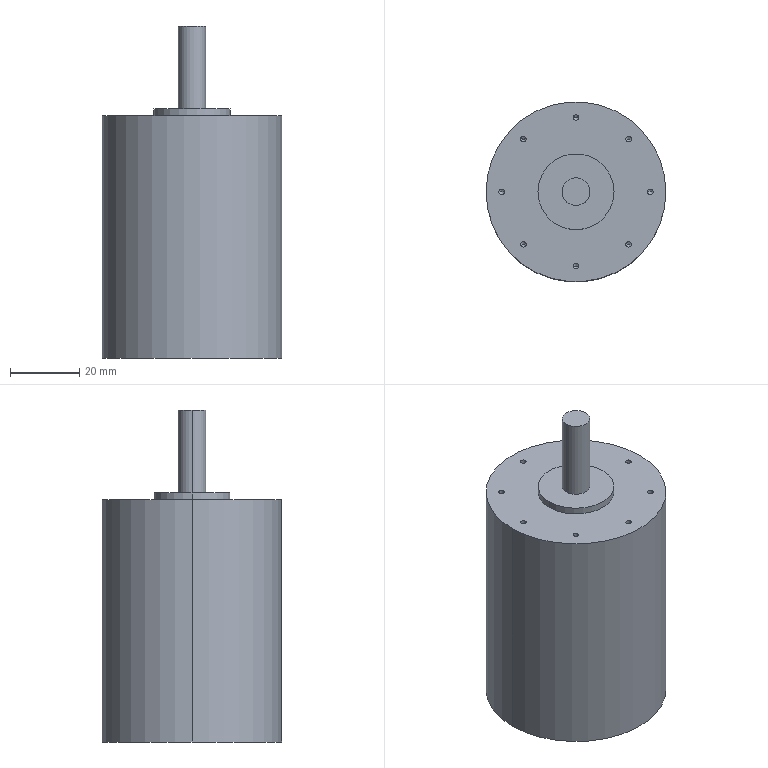Part | SolidWorks | features ICE 2, Extrusion 1, HoleWzd 1 | 1 solid | 42 faces | box 52 x 52 x 96 mm | volume 150541 mm3 | cylinder 22 | cone 16 | plane 4 | commonest cylinder face diameters 1.6 x16 8 x2 22 x2 52 x2
STEP:
#1=CARTESIAN_POINT('',(-0.8,21.5,64.8));
#2=VERTEX_POINT('',#1);
#3=CARTESIAN_POINT('',(0.8,21.5,64.8));
#4=VERTEX_POINT('',#3);
#5=CARTESIAN_POINT('',(0.,21.5,64.8));
#6=DIRECTION('',(0.,0.,1.));
#7=DIRECTION('',(1.,0.,0.));
#8=AXIS2_PLACEMENT_3D('',#5,#6,#7);
#9=CIRCLE('',#8,0.8);
#10=EDGE_CURVE('',#2,#4,#9,.T.);
#11=ORIENTED_EDGE('',*,*,#10,.F.);
#12=CARTESIAN_POINT('',(-0.8,21.5,70.));
#13=VERTEX_POINT('',#12);
#14=CARTESIAN_POINT('',(-0.8,21.5,70.));
#15=DIRECTION('',(0.,0.,1.));
#16=VECTOR('',#15,1000.);
#17=LINE('',#14,#16);
#18=EDGE_CURVE('',#2,#13,#17,.T.);
#19=ORIENTED_EDGE('',*,*,#18,.T.);
#20=CARTESIAN_POINT('',(0.8,21.5,70.));
#21=VERTEX_POINT('',#20);
#22=CARTESIAN_POINT('',(0.,21.5,70.));
#23=DIRECTION('',(0.,0.,1.));
#24=DIRECTION('',(1.,0.,0.));
#25=AXIS2_PLACEMENT_3D('',#22,#23,#24);
#26=CIRCLE('',#25,0.8);
#27=EDGE_CURVE('',#13,#21,#26,.T.);
#28=ORIENTED_EDGE('',*,*,#27,.T.);
#29=CARTESIAN_POINT('',(0.8,21.5,70.));
#30=DIRECTION('',(0.,0.,1.));
#31=VECTOR('',#30,1000.);
#32=LINE('',#29,#31);
#33=EDGE_CURVE('',#4,#21,#32,.T.);
#34=ORIENTED_EDGE('',*,*,#33,.F.);
#35=EDGE_LOOP('',(#11,#19,#28,#34));
#36=FACE_OUTER_BOUND('',#35,.T.);
#37=CARTESIAN_POINT('',(0.,21.5,70.));
#38=DIRECTION('',(0.,0.,1.));
#39=DIRECTION('',(1.,0.,0.));
#40=AXIS2_PLACEMENT_3D('',#37,#38,#39);
#41=CYLINDRICAL_SURFACE('',#40,0.8);
#42=ADVANCED_FACE('',(#36),#41,.F.);
#43=CARTESIAN_POINT('',(0.,21.5,64.319));
#44=VERTEX_POINT('',#43);
#45=CARTESIAN_POINT('',(0.8,21.5,64.8));
#46=DIRECTION('',(0.8572,0.,0.515));
#47=VECTOR('',#46,1000.);
#48=LINE('',#45,#47);
#49=EDGE_CURVE('',#44,#4,#48,.T.);
#50=ORIENTED_EDGE('',*,*,#49,.F.);
#51=CARTESIAN_POINT('',(-0.8,21.5,64.8));
#52=DIRECTION('',(-0.8572,0.,0.515));
#53=VECTOR('',#52,1000.);
#54=LINE('',#51,#53);
#55=EDGE_CURVE('',#44,#2,#54,.T.);
#56=ORIENTED_EDGE('',*,*,#55,.T.);
#57=ORIENTED_EDGE('',*,*,#10,.T.);
#58=EDGE_LOOP('',(#50,#56,#57));
#59=FACE_OUTER_BOUND('',#58,.T.);
#60=CARTESIAN_POINT('',(0.,21.5,64.8));
#61=DIRECTION('',(0.,0.,1.));
#62=DIRECTION('',(1.,0.,0.));
#63=AXIS2_PLACEMENT_3D('',#60,#61,#62);
#64=CONICAL_SURFACE('',#63,0.8,1.03);
#65=ADVANCED_FACE('',(#59),#64,.F.);
#66=CARTESIAN_POINT('',(14.403,15.203,64.8));
#67=VERTEX_POINT('',#66);
#68=CARTESIAN_POINT('',(16.003,15.203,64.8));
#69=VERTEX_POINT('',#68);
#70=CARTESIAN_POINT('',(15.203,15.203,64.8));
#71=DIRECTION('',(0.,0.,1.));
#72=DIRECTION('',(1.,0.,0.));
#73=AXIS2_PLACEMENT_3D('',#70,#71,#72);
#74=CIRCLE('',#73,0.8);
#75=EDGE_CURVE('',#67,#69,#74,.T.);
#76=ORIENTED_EDGE('',*,*,#75,.F.);
#77=CARTESIAN_POINT('',(14.403,15.203,70.));
#78=VERTEX_POINT('',#77);
#79=CARTESIAN_POINT('',(14.403,15.203,70.));
#80=DIRECTION('',(0.,0.,1.));
#81=VECTOR('',#80,1000.);
#82=LINE('',#79,#81);
#83=EDGE_CURVE('',#67,#78,#82,.T.);
#84=ORIENTED_EDGE('',*,*,#83,.T.);
#85=CARTESIAN_POINT('',(16.003,15.203,70.));
#86=VERTEX_POINT('',#85);
#87=CARTESIAN_POINT('',(15.203,15.203,70.));
#88=DIRECTION('',(0.,0.,1.));
#89=DIRECTION('',(1.,0.,0.));
#90=AXIS2_PLACEMENT_3D('',#87,#88,#89);
#91=CIRCLE('',#90,0.8);
#92=EDGE_CURVE('',#78,#86,#91,.T.);
#93=ORIENTED_EDGE('',*,*,#92,.T.);
#94=CARTESIAN_POINT('',(16.003,15.203,70.));
#95=DIRECTION('',(0.,0.,1.));
#96=VECTOR('',#95,1000.);
#97=LINE('',#94,#96);
#98=EDGE_CURVE('',#69,#86,#97,.T.);
#99=ORIENTED_EDGE('',*,*,#98,.F.);
#100=EDGE_LOOP('',(#76,#84,#93,#99));
#101=FACE_OUTER_BOUND('',#100,.T.);
#102=CARTESIAN_POINT('',(15.203,15.203,70.));
#103=DIRECTION('',(0.,0.,1.));
#104=DIRECTION('',(1.,0.,0.));
#105=AXIS2_PLACEMENT_3D('',#102,#103,#104);
#106=CYLINDRICAL_SURFACE('',#105,0.8);
#107=ADVANCED_FACE('',(#101),#106,.F.);
#108=CARTESIAN_POINT('',(15.203,15.203,64.319));
#109=VERTEX_POINT('',#108);
#110=CARTESIAN_POINT('',(16.003,15.203,64.8));
#111=DIRECTION('',(0.8572,0.,0.515));
#112=VECTOR('',#111,1000.);
#113=LINE('',#110,#112);
#114=EDGE_CURVE('',#109,#69,#113,.T.);
#115=ORIENTED_EDGE('',*,*,#114,.F.);
#116=CARTESIAN_POINT('',(14.403,15.203,64.8));
#117=DIRECTION('',(-0.8572,0.,0.515));
#118=VECTOR('',#117,1000.);
#119=LINE('',#116,#118);
#120=EDGE_CURVE('',#109,#67,#119,.T.);
#121=ORIENTED_EDGE('',*,*,#120,.T.);
#122=ORIENTED_EDGE('',*,*,#75,.T.);
#123=EDGE_LOOP('',(#115,#121,#122));
#124=FACE_OUTER_BOUND('',#123,.T.);
#125=CARTESIAN_POINT('',(15.203,15.203,64.8));
#126=DIRECTION('',(0.,0.,1.));
#127=DIRECTION('',(1.,0.,0.));
#128=AXIS2_PLACEMENT_3D('',#125,#126,#127);
#129=CONICAL_SURFACE('',#128,0.8,1.03);
#130=ADVANCED_FACE('',(#124),#129,.F.);
#131=CARTESIAN_POINT('',(20.7,0.,64.8));
#132=VERTEX_POINT('',#131);
#133=CARTESIAN_POINT('',(22.3,0.,64.8));
#134=VERTEX_POINT('',#133);
#135=CARTESIAN_POINT('',(21.5,0.,64.8));
#136=DIRECTION('',(0.,0.,1.));
#137=DIRECTION('',(1.,0.,0.));
#138=AXIS2_PLACEMENT_3D('',#135,#136,#137);
#139=CIRCLE('',#138,0.8);
#140=EDGE_CURVE('',#132,#134,#139,.T.);
#141=ORIENTED_EDGE('',*,*,#140,.F.);
#142=CARTESIAN_POINT('',(20.7,0.,70.));
#143=VERTEX_POINT('',#142);
#144=CARTESIAN_POINT('',(20.7,0.,70.));
#145=DIRECTION('',(0.,0.,1.));
#146=VECTOR('',#145,1000.);
#147=LINE('',#144,#146);
#148=EDGE_CURVE('',#132,#143,#147,.T.);
#149=ORIENTED_EDGE('',*,*,#148,.T.);
#150=CARTESIAN_POINT('',(22.3,0.,70.));
#151=VERTEX_POINT('',#150);
#152=CARTESIAN_POINT('',(21.5,0.,70.));
#153=DIRECTION('',(0.,0.,1.));
#154=DIRECTION('',(1.,0.,0.));
#155=AXIS2_PLACEMENT_3D('',#152,#153,#154);
#156=CIRCLE('',#155,0.8);
#157=EDGE_CURVE('',#143,#151,#156,.T.);
#158=ORIENTED_EDGE('',*,*,#157,.T.);
#159=CARTESIAN_POINT('',(22.3,0.,70.));
#160=DIRECTION('',(0.,0.,1.));
#161=VECTOR('',#160,1000.);
#162=LINE('',#159,#161);
#163=EDGE_CURVE('',#134,#151,#162,.T.);
#164=ORIENTED_EDGE('',*,*,#163,.F.);
#165=EDGE_LOOP('',(#141,#149,#158,#164));
#166=FACE_OUTER_BOUND('',#165,.T.);
#167=CARTESIAN_POINT('',(21.5,0.,70.));
#168=DIRECTION('',(0.,0.,1.));
#169=DIRECTION('',(1.,0.,0.));
#170=AXIS2_PLACEMENT_3D('',#167,#168,#169);
#171=CYLINDRICAL_SURFACE('',#170,0.8);
#172=ADVANCED_FACE('',(#166),#171,.F.);
#173=CARTESIAN_POINT('',(21.5,0.,64.319));
#174=VERTEX_POINT('',#173);
#175=CARTESIAN_POINT('',(22.3,0.,64.8));
#176=DIRECTION('',(0.8572,0.,0.515));
#177=VECTOR('',#176,1000.);
#178=LINE('',#175,#177);
#179=EDGE_CURVE('',#174,#134,#178,.T.);
#180=ORIENTED_EDGE('',*,*,#179,.F.);
#181=CARTESIAN_POINT('',(20.7,0.,64.8));
#182=DIRECTION('',(-0.8572,0.,0.515));
#183=VECTOR('',#182,1000.);
#184=LINE('',#181,#183);
#185=EDGE_CURVE('',#174,#132,#184,.T.);
#186=ORIENTED_EDGE('',*,*,#185,.T.);
#187=ORIENTED_EDGE('',*,*,#140,.T.);
#188=EDGE_LOOP('',(#180,#186,#187));
#189=FACE_OUTER_BOUND('',#188,.T.);
#190=CARTESIAN_POINT('',(21.5,0.,64.8));
#191=DIRECTION('',(0.,0.,1.));
#192=DIRECTION('',(1.,0.,0.));
#193=AXIS2_PLACEMENT_3D('',#190,#191,#192);
#194=CONICAL_SURFACE('',#193,0.8,1.03);
#195=ADVANCED_FACE('',(#189),#194,.F.);
#196=CARTESIAN_POINT('',(14.403,-15.203,64.8));
#197=VERTEX_POINT('',#196);
#198=CARTESIAN_POINT('',(16.003,-15.203,64.8));
#199=VERTEX_POINT('',#198);
#200=CARTESIAN_POINT('',(15.203,-15.203,64.8));
#201=DIRECTION('',(0.,0.,1.));
#202=DIRECTION('',(1.,0.,0.));
#203=AXIS2_PLACEMENT_3D('',#200,#201,#202);
#204=CIRCLE('',#203,0.8);
#205=EDGE_CURVE('',#197,#199,#204,.T.);
#206=ORIENTED_EDGE('',*,*,#205,.F.);
#207=CARTESIAN_POINT('',(14.403,-15.203,70.));
#208=VERTEX_POINT('',#207);
#209=CARTESIAN_POINT('',(14.403,-15.203,70.));
#210=DIRECTION('',(0.,0.,1.));
#211=VECTOR('',#210,1000.);
#212=LINE('',#209,#211);
#213=EDGE_CURVE('',#197,#208,#212,.T.);
#214=ORIENTED_EDGE('',*,*,#213,.T.);
#215=CARTESIAN_POINT('',(16.003,-15.203,70.));
#216=VERTEX_POINT('',#215);
#217=CARTESIAN_POINT('',(15.203,-15.203,70.));
#218=DIRECTION('',(0.,0.,1.));
#219=DIRECTION('',(1.,0.,0.));
#220=AXIS2_PLACEMENT_3D('',#217,#218,#219);
#221=CIRCLE('',#220,0.8);
#222=EDGE_CURVE('',#208,#216,#221,.T.);
#223=ORIENTED_EDGE('',*,*,#222,.T.);
#224=CARTESIAN_POINT('',(16.003,-15.203,70.));
#225=DIRECTION('',(0.,0.,1.));
#226=VECTOR('',#225,1000.);
#227=LINE('',#224,#226);
#228=EDGE_CURVE('',#199,#216,#227,.T.);
#229=ORIENTED_EDGE('',*,*,#228,.F.);
#230=EDGE_LOOP('',(#206,#214,#223,#229));
#231=FACE_OUTER_BOUND('',#230,.T.);
#232=CARTESIAN_POINT('',(15.203,-15.203,70.));
#233=DIRECTION('',(0.,0.,1.));
#234=DIRECTION('',(1.,0.,0.));
#235=AXIS2_PLACEMENT_3D('',#232,#233,#234);
#236=CYLINDRICAL_SURFACE('',#235,0.8);
#237=ADVANCED_FACE('',(#231),#236,.F.);
#238=CARTESIAN_POINT('',(15.203,-15.203,64.319));
#239=VERTEX_POINT('',#238);
#240=CARTESIAN_POINT('',(16.003,-15.203,64.8));
#241=DIRECTION('',(0.8572,0.,0.515));
#242=VECTOR('',#241,1000.);
#243=LINE('',#240,#242);
#244=EDGE_CURVE('',#239,#199,#243,.T.);
#245=ORIENTED_EDGE('',*,*,#244,.F.);
#246=CARTESIAN_POINT('',(14.403,-15.203,64.8));
#247=DIRECTION('',(-0.8572,0.,0.515));
#248=VECTOR('',#247,1000.);
#249=LINE('',#246,#248);
#250=EDGE_CURVE('',#239,#197,#249,.T.);
#251=ORIENTED_EDGE('',*,*,#250,.T.);
#252=ORIENTED_EDGE('',*,*,#205,.T.);
#253=EDGE_LOOP('',(#245,#251,#252));
#254=FACE_OUTER_BOUND('',#253,.T.);
#255=CARTESIAN_POINT('',(15.203,-15.203,64.8));
#256=DIRECTION('',(0.,0.,1.));
#257=DIRECTION('',(1.,0.,0.));
#258=AXIS2_PLACEMENT_3D('',#255,#256,#257);
#259=CONICAL_SURFACE('',#258,0.8,1.03);
#260=ADVANCED_FACE('',(#254),#259,.F.);
#261=CARTESIAN_POINT('',(-0.8,-21.5,64.8));
#262=VERTEX_POINT('',#261);
#263=CARTESIAN_POINT('',(0.8,-21.5,64.8));
#264=VERTEX_POINT('',#263);
#265=CARTESIAN_POINT('',(0.,-21.5,64.8));
#266=DIRECTION('',(0.,0.,1.));
#267=DIRECTION('',(1.,0.,0.));
#268=AXIS2_PLACEMENT_3D('',#265,#266,#267);
#269=CIRCLE('',#268,0.8);
#270=EDGE_CURVE('',#262,#264,#269,.T.);
#271=ORIENTED_EDGE('',*,*,#270,.F.);
#272=CARTESIAN_POINT('',(-0.8,-21.5,70.));
#273=VERTEX_POINT('',#272);
#274=CARTESIAN_POINT('',(-0.8,-21.5,70.));
#275=DIRECTION('',(0.,0.,1.));
#276=VECTOR('',#275,1000.);
#277=LINE('',#274,#276);
#278=EDGE_CURVE('',#262,#273,#277,.T.);
#279=ORIENTED_EDGE('',*,*,#278,.T.);
#280=CARTESIAN_POINT('',(0.8,-21.5,70.));
#281=VERTEX_POINT('',#280);
#282=CARTESIAN_POINT('',(0.,-21.5,70.));
#283=DIRECTION('',(0.,0.,1.));
#284=DIRECTION('',(1.,0.,0.));
#285=AXIS2_PLACEMENT_3D('',#282,#283,#284);
#286=CIRCLE('',#285,0.8);
#287=EDGE_CURVE('',#273,#281,#286,.T.);
#288=ORIENTED_EDGE('',*,*,#287,.T.);
#289=CARTESIAN_POINT('',(0.8,-21.5,70.));
#290=DIRECTION('',(0.,0.,1.));
#291=VECTOR('',#290,1000.);
#292=LINE('',#289,#291);
#293=EDGE_CURVE('',#264,#281,#292,.T.);
#294=ORIENTED_EDGE('',*,*,#293,.F.);
#295=EDGE_LOOP('',(#271,#279,#288,#294));
#296=FACE_OUTER_BOUND('',#295,.T.);
#297=CARTESIAN_POINT('',(0.,-21.5,70.));
#298=DIRECTION('',(0.,0.,1.));
#299=DIRECTION('',(1.,0.,0.));
#300=AXIS2_PLACEMENT_3D('',#297,#298,#299);
#301=CYLINDRICAL_SURFACE('',#300,0.8);
#302=ADVANCED_FACE('',(#296),#301,.F.);
#303=CARTESIAN_POINT('',(0.,-21.5,64.319));
#304=VERTEX_POINT('',#303);
#305=CARTESIAN_POINT('',(0.8,-21.5,64.8));
#306=DIRECTION('',(0.8572,0.,0.515));
#307=VECTOR('',#306,1000.);
#308=LINE('',#305,#307);
#309=EDGE_CURVE('',#304,#264,#308,.T.);
#310=ORIENTED_EDGE('',*,*,#309,.F.);
#311=CARTESIAN_POINT('',(-0.8,-21.5,64.8));
#312=DIRECTION('',(-0.8572,0.,0.515));
#313=VECTOR('',#312,1000.);
#314=LINE('',#311,#313);
#315=EDGE_CURVE('',#304,#262,#314,.T.);
#316=ORIENTED_EDGE('',*,*,#315,.T.);
#317=ORIENTED_EDGE('',*,*,#270,.T.);
#318=EDGE_LOOP('',(#310,#316,#317));
#319=FACE_OUTER_BOUND('',#318,.T.);
#320=CARTESIAN_POINT('',(0.,-21.5,64.8));
#321=DIRECTION('',(0.,0.,1.));
#322=DIRECTION('',(1.,0.,0.));
#323=AXIS2_PLACEMENT_3D('',#320,#321,#322);
#324=CONICAL_SURFACE('',#323,0.8,1.03);
#325=ADVANCED_FACE('',(#319),#324,.F.);
#326=CARTESIAN_POINT('',(-16.003,-15.203,64.8));
#327=VERTEX_POINT('',#326);
#328=CARTESIAN_POINT('',(-14.403,-15.203,64.8));
#329=VERTEX_POINT('',#328);
#330=CARTESIAN_POINT('',(-15.203,-15.203,64.8));
#331=DIRECTION('',(0.,0.,1.));
#332=DIRECTION('',(1.,0.,0.));
#333=AXIS2_PLACEMENT_3D('',#330,#331,#332);
#334=CIRCLE('',#333,0.8);
#335=EDGE_CURVE('',#327,#329,#334,.T.);
#336=ORIENTED_EDGE('',*,*,#335,.F.);
#337=CARTESIAN_POINT('',(-16.003,-15.203,70.));
#338=VERTEX_POINT('',#337);
#339=CARTESIAN_POINT('',(-16.003,-15.203,70.));
#340=DIRECTION('',(0.,0.,1.));
#341=VECTOR('',#340,1000.);
#342=LINE('',#339,#341);
#343=EDGE_CURVE('',#327,#338,#342,.T.);
#344=ORIENTED_EDGE('',*,*,#343,.T.);
#345=CARTESIAN_POINT('',(-14.403,-15.203,70.));
#346=VERTEX_POINT('',#345);
#347=CARTESIAN_POINT('',(-15.203,-15.203,70.));
#348=DIRECTION('',(0.,0.,1.));
#349=DIRECTION('',(1.,0.,0.));
#350=AXIS2_PLACEMENT_3D('',#347,#348,#349);
#351=CIRCLE('',#350,0.8);
#352=EDGE_CURVE('',#338,#346,#351,.T.);
#353=ORIENTED_EDGE('',*,*,#352,.T.);
#354=CARTESIAN_POINT('',(-14.403,-15.203,70.));
#355=DIRECTION('',(0.,0.,1.));
#356=VECTOR('',#355,1000.);
#357=LINE('',#354,#356);
#358=EDGE_CURVE('',#329,#346,#357,.T.);
#359=ORIENTED_EDGE('',*,*,#358,.F.);
#360=EDGE_LOOP('',(#336,#344,#353,#359));
#361=FACE_OUTER_BOUND('',#360,.T.);
#362=CARTESIAN_POINT('',(-15.203,-15.203,70.));
#363=DIRECTION('',(0.,0.,1.));
#364=DIRECTION('',(1.,0.,0.));
#365=AXIS2_PLACEMENT_3D('',#362,#363,#364);
#366=CYLINDRICAL_SURFACE('',#365,0.8);
#367=ADVANCED_FACE('',(#361),#366,.F.);
#368=CARTESIAN_POINT('',(-15.203,-15.203,64.319));
#369=VERTEX_POINT('',#368);
#370=CARTESIAN_POINT('',(-14.403,-15.203,64.8));
#371=DIRECTION('',(0.8572,0.,0.515));
#372=VECTOR('',#371,1000.);
#373=LINE('',#370,#372);
#374=EDGE_CURVE('',#369,#329,#373,.T.);
#375=ORIENTED_EDGE('',*,*,#374,.F.);
#376=CARTESIAN_POINT('',(-16.003,-15.203,64.8));
#377=DIRECTION('',(-0.8572,0.,0.515));
#378=VECTOR('',#377,1000.);
#379=LINE('',#376,#378);
#380=EDGE_CURVE('',#369,#327,#379,.T.);
#381=ORIENTED_EDGE('',*,*,#380,.T.);
#382=ORIENTED_EDGE('',*,*,#335,.T.);
#383=EDGE_LOOP('',(#375,#381,#382));
#384=FACE_OUTER_BOUND('',#383,.T.);
#385=CARTESIAN_POINT('',(-15.203,-15.203,64.8));
#386=DIRECTION('',(0.,0.,1.));
#387=DIRECTION('',(1.,0.,0.));
#388=AXIS2_PLACEMENT_3D('',#385,#386,#387);
#389=CONICAL_SURFACE('',#388,0.8,1.03);
#390=ADVANCED_FACE('',(#384),#389,.F.);
#391=CARTESIAN_POINT('',(-22.3,0.,64.8));
#392=VERTEX_POINT('',#391);
#393=CARTESIAN_POINT('',(-20.7,0.,64.8));
#394=VERTEX_POINT('',#393);
#395=CARTESIAN_POINT('',(-21.5,0.,64.8));
#396=DIRECTION('',(0.,0.,1.));
#397=DIRECTION('',(1.,0.,0.));
#398=AXIS2_PLACEMENT_3D('',#395,#396,#397);
#399=CIRCLE('',#398,0.8);
#400=EDGE_CURVE('',#392,#394,#399,.T.);
#401=ORIENTED_EDGE('',*,*,#400,.F.);
#402=CARTESIAN_POINT('',(-22.3,0.,70.));
#403=VERTEX_POINT('',#402);
#404=CARTESIAN_POINT('',(-22.3,0.,70.));
#405=DIRECTION('',(0.,0.,1.));
#406=VECTOR('',#405,1000.);
#407=LINE('',#404,#406);
#408=EDGE_CURVE('',#392,#403,#407,.T.);
#409=ORIENTED_EDGE('',*,*,#408,.T.);
#410=CARTESIAN_POINT('',(-20.7,0.,70.));
#411=VERTEX_POINT('',#410);
#412=CARTESIAN_POINT('',(-21.5,0.,70.));
#413=DIRECTION('',(0.,0.,1.));
#414=DIRECTION('',(1.,0.,0.));
#415=AXIS2_PLACEMENT_3D('',#412,#413,#414);
#416=CIRCLE('',#415,0.8);
#417=EDGE_CURVE('',#403,#411,#416,.T.);
#418=ORIENTED_EDGE('',*,*,#417,.T.);
#419=CARTESIAN_POINT('',(-20.7,0.,70.));
#420=DIRECTION('',(0.,0.,1.));
#421=VECTOR('',#420,1000.);
#422=LINE('',#419,#421);
#423=EDGE_CURVE('',#394,#411,#422,.T.);
#424=ORIENTED_EDGE('',*,*,#423,.F.);
#425=EDGE_LOOP('',(#401,#409,#418,#424));
#426=FACE_OUTER_BOUND('',#425,.T.);
#427=CARTESIAN_POINT('',(-21.5,0.,70.));
#428=DIRECTION('',(0.,0.,1.));
#429=DIRECTION('',(1.,0.,0.));
#430=AXIS2_PLACEMENT_3D('',#427,#428,#429);
#431=CYLINDRICAL_SURFACE('',#430,0.8);
#432=ADVANCED_FACE('',(#426),#431,.F.);
#433=CARTESIAN_POINT('',(-21.5,0.,64.319));
#434=VERTEX_POINT('',#433);
#435=CARTESIAN_POINT('',(-20.7,0.,64.8));
#436=DIRECTION('',(0.8572,0.,0.515));
#437=VECTOR('',#436,1000.);
#438=LINE('',#435,#437);
#439=EDGE_CURVE('',#434,#394,#438,.T.);
#440=ORIENTED_EDGE('',*,*,#439,.F.);
#441=CARTESIAN_POINT('',(-22.3,0.,64.8));
#442=DIRECTION('',(-0.8572,0.,0.515));
#443=VECTOR('',#442,1000.);
#444=LINE('',#441,#443);
#445=EDGE_CURVE('',#434,#392,#444,.T.);
#446=ORIENTED_EDGE('',*,*,#445,.T.);
#447=ORIENTED_EDGE('',*,*,#400,.T.);
#448=EDGE_LOOP('',(#440,#446,#447));
#449=FACE_OUTER_BOUND('',#448,.T.);
#450=CARTESIAN_POINT('',(-21.5,0.,64.8));
#451=DIRECTION('',(0.,0.,1.));
#452=DIRECTION('',(1.,0.,0.));
#453=AXIS2_PLACEMENT_3D('',#450,#451,#452);
#454=CONICAL_SURFACE('',#453,0.8,1.03);
#455=ADVANCED_FACE('',(#449),#454,.F.);
#456=CARTESIAN_POINT('',(-16.003,15.203,64.8));
#457=VERTEX_POINT('',#456);
#458=CARTESIAN_POINT('',(-14.403,15.203,64.8));
#459=VERTEX_POINT('',#458);
#460=CARTESIAN_POINT('',(-15.203,15.203,64.8));
#461=DIRECTION('',(0.,0.,1.));
#462=DIRECTION('',(1.,0.,0.));
#463=AXIS2_PLACEMENT_3D('',#460,#461,#462);
#464=CIRCLE('',#463,0.8);
#465=EDGE_CURVE('',#457,#459,#464,.T.);
#466=ORIENTED_EDGE('',*,*,#465,.F.);
#467=CARTESIAN_POINT('',(-16.003,15.203,70.));
#468=VERTEX_POINT('',#467);
#469=CARTESIAN_POINT('',(-16.003,15.203,70.));
#470=DIRECTION('',(0.,0.,1.));
#471=VECTOR('',#470,1000.);
#472=LINE('',#469,#471);
#473=EDGE_CURVE('',#457,#468,#472,.T.);
#474=ORIENTED_EDGE('',*,*,#473,.T.);
#475=CARTESIAN_POINT('',(-14.403,15.203,70.));
#476=VERTEX_POINT('',#475);
#477=CARTESIAN_POINT('',(-15.203,15.203,70.));
#478=DIRECTION('',(0.,0.,1.));
#479=DIRECTION('',(1.,0.,0.));
#480=AXIS2_PLACEMENT_3D('',#477,#478,#479);
#481=CIRCLE('',#480,0.8);
#482=EDGE_CURVE('',#468,#476,#481,.T.);
#483=ORIENTED_EDGE('',*,*,#482,.T.);
#484=CARTESIAN_POINT('',(-14.403,15.203,70.));
#485=DIRECTION('',(0.,0.,1.));
#486=VECTOR('',#485,1000.);
#487=LINE('',#484,#486);
#488=EDGE_CURVE('',#459,#476,#487,.T.);
#489=ORIENTED_EDGE('',*,*,#488,.F.);
#490=EDGE_LOOP('',(#466,#474,#483,#489));
#491=FACE_OUTER_BOUND('',#490,.T.);
#492=CARTESIAN_POINT('',(-15.203,15.203,70.));
#493=DIRECTION('',(0.,0.,1.));
#494=DIRECTION('',(1.,0.,0.));
#495=AXIS2_PLACEMENT_3D('',#492,#493,#494);
#496=CYLINDRICAL_SURFACE('',#495,0.8);
#497=ADVANCED_FACE('',(#491),#496,.F.);
#498=CARTESIAN_POINT('',(-15.203,15.203,64.319));
#499=VERTEX_POINT('',#498);
#500=CARTESIAN_POINT('',(-14.403,15.203,64.8));
#501=DIRECTION('',(0.8572,0.,0.515));
#502=VECTOR('',#501,1000.);
#503=LINE('',#500,#502);
#504=EDGE_CURVE('',#499,#459,#503,.T.);
#505=ORIENTED_EDGE('',*,*,#504,.F.);
#506=CARTESIAN_POINT('',(-16.003,15.203,64.8));
#507=DIRECTION('',(-0.8572,0.,0.515));
#508=VECTOR('',#507,1000.);
#509=LINE('',#506,#508);
#510=EDGE_CURVE('',#499,#457,#509,.T.);
#511=ORIENTED_EDGE('',*,*,#510,.T.);
#512=ORIENTED_EDGE('',*,*,#465,.T.);
#513=EDGE_LOOP('',(#505,#511,#512));
#514=FACE_OUTER_BOUND('',#513,.T.);
#515=CARTESIAN_POINT('',(-15.203,15.203,64.8));
#516=DIRECTION('',(0.,0.,1.));
#517=DIRECTION('',(1.,0.,0.));
#518=AXIS2_PLACEMENT_3D('',#515,#516,#517);
#519=CONICAL_SURFACE('',#518,0.8,1.03);
#520=ADVANCED_FACE('',(#514),#519,.F.);
#521=CARTESIAN_POINT('',(4.,0.,96.));
#522=VERTEX_POINT('',#521);
#523=CARTESIAN_POINT('',(-4.,0.,96.));
#524=VERTEX_POINT('',#523);
#525=CARTESIAN_POINT('',(0.,0.,96.));
#526=DIRECTION('',(0.,0.,1.));
#527=DIRECTION('',(1.,0.,0.));
#528=AXIS2_PLACEMENT_3D('',#525,#526,#527);
#529=CIRCLE('',#528,4.);
#530=EDGE_CURVE('',#522,#524,#529,.T.);
#531=ORIENTED_EDGE('',*,*,#530,.F.);
#532=CARTESIAN_POINT('',(4.,0.,72.));
#533=VERTEX_POINT('',#532);
#534=CARTESIAN_POINT('',(4.,0.,96.));
#535=DIRECTION('',(0.,0.,-1.));
#536=VECTOR('',#535,1000.);
#537=LINE('',#534,#536);
#538=EDGE_CURVE('',#522,#533,#537,.T.);
#539=ORIENTED_EDGE('',*,*,#538,.T.);
#540=CARTESIAN_POINT('',(-4.,0.,72.));
#541=VERTEX_POINT('',#540);
#542=CARTESIAN_POINT('',(0.,0.,72.));
#543=DIRECTION('',(0.,0.,1.));
#544=DIRECTION('',(1.,0.,0.));
#545=AXIS2_PLACEMENT_3D('',#542,#543,#544);
#546=CIRCLE('',#545,4.);
#547=EDGE_CURVE('',#533,#541,#546,.T.);
#548=ORIENTED_EDGE('',*,*,#547,.T.);
#549=CARTESIAN_POINT('',(-4.,0.,96.));
#550=DIRECTION('',(0.,0.,-1.));
#551=VECTOR('',#550,1000.);
#552=LINE('',#549,#551);
#553=EDGE_CURVE('',#524,#541,#552,.T.);
#554=ORIENTED_EDGE('',*,*,#553,.F.);
#555=EDGE_LOOP('',(#531,#539,#548,#554));
#556=FACE_OUTER_BOUND('',#555,.T.);
#557=CARTESIAN_POINT('',(0.,0.,96.));
#558=DIRECTION('',(0.,0.,-1.));
#559=DIRECTION('',(-1.,0.,0.));
#560=AXIS2_PLACEMENT_3D('',#557,#558,#559);
#561=CYLINDRICAL_SURFACE('',#560,4.);
#562=ADVANCED_FACE('',(#556),#561,.T.);
#563=CARTESIAN_POINT('',(11.,0.,72.));
#564=VERTEX_POINT('',#563);
#565=CARTESIAN_POINT('',(-11.,0.,72.));
#566=VERTEX_POINT('',#565);
#567=CARTESIAN_POINT('',(0.,0.,72.));
#568=DIRECTION('',(0.,0.,1.));
#569=DIRECTION('',(1.,0.,0.));
#570=AXIS2_PLACEMENT_3D('',#567,#568,#569);
#571=CIRCLE('',#570,11.);
#572=EDGE_CURVE('',#564,#566,#571,.T.);
#573=ORIENTED_EDGE('',*,*,#572,.F.);
#574=CARTESIAN_POINT('',(11.,0.,70.));
#575=VERTEX_POINT('',#574);
#576=CARTESIAN_POINT('',(11.,0.,72.));
#577=DIRECTION('',(0.,0.,-1.));
#578=VECTOR('',#577,1000.);
#579=LINE('',#576,#578);
#580=EDGE_CURVE('',#564,#575,#579,.T.);
#581=ORIENTED_EDGE('',*,*,#580,.T.);
#582=CARTESIAN_POINT('',(-11.,0.,70.));
#583=VERTEX_POINT('',#582);
#584=CARTESIAN_POINT('',(0.,0.,70.));
#585=DIRECTION('',(0.,0.,1.));
#586=DIRECTION('',(1.,0.,0.));
#587=AXIS2_PLACEMENT_3D('',#584,#585,#586);
#588=CIRCLE('',#587,11.);
#589=EDGE_CURVE('',#575,#583,#588,.T.);
#590=ORIENTED_EDGE('',*,*,#589,.T.);
#591=CARTESIAN_POINT('',(-11.,0.,72.));
#592=DIRECTION('',(0.,0.,-1.));
#593=VECTOR('',#592,1000.);
#594=LINE('',#591,#593);
#595=EDGE_CURVE('',#566,#583,#594,.T.);
#596=ORIENTED_EDGE('',*,*,#595,.F.);
#597=EDGE_LOOP('',(#573,#581,#590,#596));
#598=FACE_OUTER_BOUND('',#597,.T.);
#599=CARTESIAN_POINT('',(0.,0.,72.));
#600=DIRECTION('',(0.,0.,-1.));
#601=DIRECTION('',(-1.,0.,0.));
#602=AXIS2_PLACEMENT_3D('',#599,#600,#601);
#603=CYLINDRICAL_SURFACE('',#602,11.);
#604=ADVANCED_FACE('',(#598),#603,.T.);
#605=CARTESIAN_POINT('',(26.,0.,70.));
#606=VERTEX_POINT('',#605);
#607=CARTESIAN_POINT('',(-26.,0.,70.));
#608=VERTEX_POINT('',#607);
#609=CARTESIAN_POINT('',(0.,0.,70.));
#610=DIRECTION('',(0.,0.,1.));
#611=DIRECTION('',(1.,0.,0.));
#612=AXIS2_PLACEMENT_3D('',#609,#610,#611);
#613=CIRCLE('',#612,26.);
#614=EDGE_CURVE('',#606,#608,#613,.T.);
#615=ORIENTED_EDGE('',*,*,#614,.F.);
#616=CARTESIAN_POINT('',(26.,0.,0.));
#617=VERTEX_POINT('',#616);
#618=CARTESIAN_POINT('',(26.,0.,70.));
#619=DIRECTION('',(0.,0.,-1.));
#620=VECTOR('',#619,1000.);
#621=LINE('',#618,#620);
#622=EDGE_CURVE('',#606,#617,#621,.T.);
#623=ORIENTED_EDGE('',*,*,#622,.T.);
#624=CARTESIAN_POINT('',(-26.,0.,0.));
#625=VERTEX_POINT('',#624);
#626=CARTESIAN_POINT('',(0.,0.,0.));
#627=DIRECTION('',(0.,0.,1.));
#628=DIRECTION('',(1.,0.,0.));
#629=AXIS2_PLACEMENT_3D('',#626,#627,#628);
#630=CIRCLE('',#629,26.);
#631=EDGE_CURVE('',#617,#625,#630,.T.);
#632=ORIENTED_EDGE('',*,*,#631,.T.);
#633=CARTESIAN_POINT('',(-26.,0.,70.));
#634=DIRECTION('',(0.,0.,-1.));
#635=VECTOR('',#634,1000.);
#636=LINE('',#633,#635);
#637=EDGE_CURVE('',#608,#625,#636,.T.);
#638=ORIENTED_EDGE('',*,*,#637,.F.);
#639=EDGE_LOOP('',(#615,#623,#632,#638));
#640=FACE_OUTER_BOUND('',#639,.T.);
#641=CARTESIAN_POINT('',(0.,0.,70.));
#642=DIRECTION('',(0.,0.,-1.));
#643=DIRECTION('',(-1.,0.,0.));
#644=AXIS2_PLACEMENT_3D('',#641,#642,#643);
#645=CYLINDRICAL_SURFACE('',#644,26.);
#646=ADVANCED_FACE('',(#640),#645,.T.);
#647=ORIENTED_EDGE('',*,*,#622,.F.);
#648=CARTESIAN_POINT('',(0.,0.,70.));
#649=DIRECTION('',(0.,0.,1.));
#650=DIRECTION('',(1.,0.,0.));
#651=AXIS2_PLACEMENT_3D('',#648,#649,#650);
#652=CIRCLE('',#651,26.);
#653=EDGE_CURVE('',#608,#606,#652,.T.);
#654=ORIENTED_EDGE('',*,*,#653,.F.);
#655=ORIENTED_EDGE('',*,*,#637,.T.);
#656=CARTESIAN_POINT('',(0.,0.,0.));
#657=DIRECTION('',(0.,0.,1.));
#658=DIRECTION('',(1.,0.,0.));
#659=AXIS2_PLACEMENT_3D('',#656,#657,#658);
#660=CIRCLE('',#659,26.);
#661=EDGE_CURVE('',#625,#617,#660,.T.);
#662=ORIENTED_EDGE('',*,*,#661,.T.);
#663=EDGE_LOOP('',(#647,#654,#655,#662));
#664=FACE_OUTER_BOUND('',#663,.T.);
#665=CARTESIAN_POINT('',(0.,0.,70.));
#666=DIRECTION('',(0.,0.,-1.));
#667=DIRECTION('',(-1.,0.,0.));
#668=AXIS2_PLACEMENT_3D('',#665,#666,#667);
#669=CYLINDRICAL_SURFACE('',#668,26.);
#670=ADVANCED_FACE('',(#664),#669,.T.);
#671=CARTESIAN_POINT('',(0.,21.5,70.));
#672=DIRECTION('',(0.,0.,1.));
#673=DIRECTION('',(1.,0.,0.));
#674=AXIS2_PLACEMENT_3D('',#671,#672,#673);
#675=CIRCLE('',#674,0.8);
#676=EDGE_CURVE('',#21,#13,#675,.T.);
#677=ORIENTED_EDGE('',*,*,#676,.F.);
#678=ORIENTED_EDGE('',*,*,#27,.F.);
#679=EDGE_LOOP('',(#677,#678));
#680=FACE_BOUND('',#679,.T.);
#681=CARTESIAN_POINT('',(15.203,15.203,70.));
#682=DIRECTION('',(0.,0.,1.));
#683=DIRECTION('',(1.,0.,0.));
#684=AXIS2_PLACEMENT_3D('',#681,#682,#683);
#685=CIRCLE('',#684,0.8);
#686=EDGE_CURVE('',#86,#78,#685,.T.);
#687=ORIENTED_EDGE('',*,*,#686,.F.);
#688=ORIENTED_EDGE('',*,*,#92,.F.);
#689=EDGE_LOOP('',(#687,#688));
#690=FACE_BOUND('',#689,.T.);
#691=CARTESIAN_POINT('',(21.5,0.,70.));
#692=DIRECTION('',(0.,0.,1.));
#693=DIRECTION('',(1.,0.,0.));
#694=AXIS2_PLACEMENT_3D('',#691,#692,#693);
#695=CIRCLE('',#694,0.8);
#696=EDGE_CURVE('',#151,#143,#695,.T.);
#697=ORIENTED_EDGE('',*,*,#696,.F.);
#698=ORIENTED_EDGE('',*,*,#157,.F.);
#699=EDGE_LOOP('',(#697,#698));
#700=FACE_BOUND('',#699,.T.);
#701=CARTESIAN_POINT('',(15.203,-15.203,70.));
#702=DIRECTION('',(0.,0.,1.));
#703=DIRECTION('',(1.,0.,0.));
#704=AXIS2_PLACEMENT_3D('',#701,#702,#703);
#705=CIRCLE('',#704,0.8);
#706=EDGE_CURVE('',#216,#208,#705,.T.);
#707=ORIENTED_EDGE('',*,*,#706,.F.);
#708=ORIENTED_EDGE('',*,*,#222,.F.);
#709=EDGE_LOOP('',(#707,#708));
#710=FACE_BOUND('',#709,.T.);
#711=CARTESIAN_POINT('',(0.,-21.5,70.));
#712=DIRECTION('',(0.,0.,1.));
#713=DIRECTION('',(1.,0.,0.));
#714=AXIS2_PLACEMENT_3D('',#711,#712,#713);
#715=CIRCLE('',#714,0.8);
#716=EDGE_CURVE('',#281,#273,#715,.T.);
#717=ORIENTED_EDGE('',*,*,#716,.F.);
#718=ORIENTED_EDGE('',*,*,#287,.F.);
#719=EDGE_LOOP('',(#717,#718));
#720=FACE_BOUND('',#719,.T.);
#721=CARTESIAN_POINT('',(-15.203,-15.203,70.));
#722=DIRECTION('',(0.,0.,1.));
#723=DIRECTION('',(1.,0.,0.));
#724=AXIS2_PLACEMENT_3D('',#721,#722,#723);
#725=CIRCLE('',#724,0.8);
#726=EDGE_CURVE('',#346,#338,#725,.T.);
#727=ORIENTED_EDGE('',*,*,#726,.F.);
#728=ORIENTED_EDGE('',*,*,#352,.F.);
#729=EDGE_LOOP('',(#727,#728));
#730=FACE_BOUND('',#729,.T.);
#731=CARTESIAN_POINT('',(-21.5,0.,70.));
#732=DIRECTION('',(0.,0.,1.));
#733=DIRECTION('',(1.,0.,0.));
#734=AXIS2_PLACEMENT_3D('',#731,#732,#733);
#735=CIRCLE('',#734,0.8);
#736=EDGE_CURVE('',#411,#403,#735,.T.);
#737=ORIENTED_EDGE('',*,*,#736,.F.);
#738=ORIENTED_EDGE('',*,*,#417,.F.);
#739=EDGE_LOOP('',(#737,#738));
#740=FACE_BOUND('',#739,.T.);
#741=CARTESIAN_POINT('',(-15.203,15.203,70.));
#742=DIRECTION('',(0.,0.,1.));
#743=DIRECTION('',(1.,0.,0.));
#744=AXIS2_PLACEMENT_3D('',#741,#742,#743);
#745=CIRCLE('',#744,0.8);
#746=EDGE_CURVE('',#476,#468,#745,.T.);
#747=ORIENTED_EDGE('',*,*,#746,.F.);
#748=ORIENTED_EDGE('',*,*,#482,.F.);
#749=EDGE_LOOP('',(#747,#748));
#750=FACE_BOUND('',#749,.T.);
#751=CARTESIAN_POINT('',(0.,0.,70.));
#752=DIRECTION('',(0.,0.,1.));
#753=DIRECTION('',(1.,0.,0.));
#754=AXIS2_PLACEMENT_3D('',#751,#752,#753);
#755=CIRCLE('',#754,11.);
#756=EDGE_CURVE('',#583,#575,#755,.T.);
#757=ORIENTED_EDGE('',*,*,#756,.F.);
#758=ORIENTED_EDGE('',*,*,#589,.F.);
#759=EDGE_LOOP('',(#757,#758));
#760=FACE_BOUND('',#759,.T.);
#761=ORIENTED_EDGE('',*,*,#653,.T.);
#762=ORIENTED_EDGE('',*,*,#614,.T.);
#763=EDGE_LOOP('',(#761,#762));
#764=FACE_OUTER_BOUND('',#763,.T.);
#765=CARTESIAN_POINT('',(0.,0.,70.));
#766=DIRECTION('',(0.,0.,1.));
#767=DIRECTION('',(1.,0.,0.));
#768=AXIS2_PLACEMENT_3D('',#765,#766,#767);
#769=PLANE('',#768);
#770=ADVANCED_FACE('',(#680,#690,#700,#710,#720,#730,#740,#750,#760,#764),#769,.T.);
#771=ORIENTED_EDGE('',*,*,#661,.F.);
#772=ORIENTED_EDGE('',*,*,#631,.F.);
#773=EDGE_LOOP('',(#771,#772));
#774=FACE_OUTER_BOUND('',#773,.T.);
#775=CARTESIAN_POINT('',(0.,0.,0.));
#776=DIRECTION('',(0.,0.,1.));
#777=DIRECTION('',(1.,0.,0.));
#778=AXIS2_PLACEMENT_3D('',#775,#776,#777);
#779=PLANE('',#778);
#780=ADVANCED_FACE('',(#774),#779,.F.);
#781=ORIENTED_EDGE('',*,*,#580,.F.);
#782=CARTESIAN_POINT('',(0.,0.,72.));
#783=DIRECTION('',(0.,0.,1.));
#784=DIRECTION('',(1.,0.,0.));
#785=AXIS2_PLACEMENT_3D('',#782,#783,#784);
#786=CIRCLE('',#785,11.);
#787=EDGE_CURVE('',#566,#564,#786,.T.);
#788=ORIENTED_EDGE('',*,*,#787,.F.);
#789=ORIENTED_EDGE('',*,*,#595,.T.);
#790=ORIENTED_EDGE('',*,*,#756,.T.);
#791=EDGE_LOOP('',(#781,#788,#789,#790));
#792=FACE_OUTER_BOUND('',#791,.T.);
#793=CARTESIAN_POINT('',(0.,0.,72.));
#794=DIRECTION('',(0.,0.,-1.));
#795=DIRECTION('',(-1.,0.,0.));
#796=AXIS2_PLACEMENT_3D('',#793,#794,#795);
#797=CYLINDRICAL_SURFACE('',#796,11.);
#798=ADVANCED_FACE('',(#792),#797,.T.);
#799=CARTESIAN_POINT('',(0.,0.,72.));
#800=DIRECTION('',(0.,0.,1.));
#801=DIRECTION('',(1.,0.,0.));
#802=AXIS2_PLACEMENT_3D('',#799,#800,#801);
#803=CIRCLE('',#802,4.);
#804=EDGE_CURVE('',#541,#533,#803,.T.);
#805=ORIENTED_EDGE('',*,*,#804,.F.);
#806=ORIENTED_EDGE('',*,*,#547,.F.);
#807=EDGE_LOOP('',(#805,#806));
#808=FACE_BOUND('',#807,.T.);
#809=ORIENTED_EDGE('',*,*,#787,.T.);
#810=ORIENTED_EDGE('',*,*,#572,.T.);
#811=EDGE_LOOP('',(#809,#810));
#812=FACE_OUTER_BOUND('',#811,.T.);
#813=CARTESIAN_POINT('',(0.,0.,72.));
#814=DIRECTION('',(0.,0.,1.));
#815=DIRECTION('',(1.,0.,0.));
#816=AXIS2_PLACEMENT_3D('',#813,#814,#815);
#817=PLANE('',#816);
#818=ADVANCED_FACE('',(#808,#812),#817,.T.);
#819=ORIENTED_EDGE('',*,*,#538,.F.);
#820=CARTESIAN_POINT('',(0.,0.,96.));
#821=DIRECTION('',(0.,0.,1.));
#822=DIRECTION('',(1.,0.,0.));
#823=AXIS2_PLACEMENT_3D('',#820,#821,#822);
#824=CIRCLE('',#823,4.);
#825=EDGE_CURVE('',#524,#522,#824,.T.);
#826=ORIENTED_EDGE('',*,*,#825,.F.);
#827=ORIENTED_EDGE('',*,*,#553,.T.);
#828=ORIENTED_EDGE('',*,*,#804,.T.);
#829=EDGE_LOOP('',(#819,#826,#827,#828));
#830=FACE_OUTER_BOUND('',#829,.T.);
#831=CARTESIAN_POINT('',(0.,0.,96.));
#832=DIRECTION('',(0.,0.,-1.));
#833=DIRECTION('',(-1.,0.,0.));
#834=AXIS2_PLACEMENT_3D('',#831,#832,#833);
#835=CYLINDRICAL_SURFACE('',#834,4.);
#836=ADVANCED_FACE('',(#830),#835,.T.);
#837=ORIENTED_EDGE('',*,*,#825,.T.);
#838=ORIENTED_EDGE('',*,*,#530,.T.);
#839=EDGE_LOOP('',(#837,#838));
#840=FACE_OUTER_BOUND('',#839,.T.);
#841=CARTESIAN_POINT('',(0.,0.,96.));
#842=DIRECTION('',(0.,0.,1.));
#843=DIRECTION('',(1.,0.,0.));
#844=AXIS2_PLACEMENT_3D('',#841,#842,#843);
#845=PLANE('',#844);
#846=ADVANCED_FACE('',(#840),#845,.T.);
#847=ORIENTED_EDGE('',*,*,#510,.F.);
#848=ORIENTED_EDGE('',*,*,#504,.T.);
#849=CARTESIAN_POINT('',(-15.203,15.203,64.8));
#850=DIRECTION('',(0.,0.,1.));
#851=DIRECTION('',(1.,0.,0.));
#852=AXIS2_PLACEMENT_3D('',#849,#850,#851);
#853=CIRCLE('',#852,0.8);
#854=EDGE_CURVE('',#459,#457,#853,.T.);
#855=ORIENTED_EDGE('',*,*,#854,.T.);
#856=EDGE_LOOP('',(#847,#848,#855));
#857=FACE_OUTER_BOUND('',#856,.T.);
#858=CARTESIAN_POINT('',(-15.203,15.203,64.8));
#859=DIRECTION('',(0.,0.,1.));
#860=DIRECTION('',(1.,0.,0.));
#861=AXIS2_PLACEMENT_3D('',#858,#859,#860);
#862=CONICAL_SURFACE('',#861,0.8,1.03);
#863=ADVANCED_FACE('',(#857),#862,.F.);
#864=ORIENTED_EDGE('',*,*,#473,.F.);
#865=ORIENTED_EDGE('',*,*,#854,.F.);
#866=ORIENTED_EDGE('',*,*,#488,.T.);
#867=ORIENTED_EDGE('',*,*,#746,.T.);
#868=EDGE_LOOP('',(#864,#865,#866,#867));
#869=FACE_OUTER_BOUND('',#868,.T.);
#870=CARTESIAN_POINT('',(-15.203,15.203,70.));
#871=DIRECTION('',(0.,0.,1.));
#872=DIRECTION('',(1.,0.,0.));
#873=AXIS2_PLACEMENT_3D('',#870,#871,#872);
#874=CYLINDRICAL_SURFACE('',#873,0.8);
#875=ADVANCED_FACE('',(#869),#874,.F.);
#876=ORIENTED_EDGE('',*,*,#445,.F.);
#877=ORIENTED_EDGE('',*,*,#439,.T.);
#878=CARTESIAN_POINT('',(-21.5,0.,64.8));
#879=DIRECTION('',(0.,0.,1.));
#880=DIRECTION('',(1.,0.,0.));
#881=AXIS2_PLACEMENT_3D('',#878,#879,#880);
#882=CIRCLE('',#881,0.8);
#883=EDGE_CURVE('',#394,#392,#882,.T.);
#884=ORIENTED_EDGE('',*,*,#883,.T.);
#885=EDGE_LOOP('',(#876,#877,#884));
#886=FACE_OUTER_BOUND('',#885,.T.);
#887=CARTESIAN_POINT('',(-21.5,0.,64.8));
#888=DIRECTION('',(0.,0.,1.));
#889=DIRECTION('',(1.,0.,0.));
#890=AXIS2_PLACEMENT_3D('',#887,#888,#889);
#891=CONICAL_SURFACE('',#890,0.8,1.03);
#892=ADVANCED_FACE('',(#886),#891,.F.);
#893=ORIENTED_EDGE('',*,*,#408,.F.);
#894=ORIENTED_EDGE('',*,*,#883,.F.);
#895=ORIENTED_EDGE('',*,*,#423,.T.);
#896=ORIENTED_EDGE('',*,*,#736,.T.);
#897=EDGE_LOOP('',(#893,#894,#895,#896));
#898=FACE_OUTER_BOUND('',#897,.T.);
#899=CARTESIAN_POINT('',(-21.5,0.,70.));
#900=DIRECTION('',(0.,0.,1.));
#901=DIRECTION('',(1.,0.,0.));
#902=AXIS2_PLACEMENT_3D('',#899,#900,#901);
#903=CYLINDRICAL_SURFACE('',#902,0.8);
#904=ADVANCED_FACE('',(#898),#903,.F.);
#905=ORIENTED_EDGE('',*,*,#380,.F.);
#906=ORIENTED_EDGE('',*,*,#374,.T.);
#907=CARTESIAN_POINT('',(-15.203,-15.203,64.8));
#908=DIRECTION('',(0.,0.,1.));
#909=DIRECTION('',(1.,0.,0.));
#910=AXIS2_PLACEMENT_3D('',#907,#908,#909);
#911=CIRCLE('',#910,0.8);
#912=EDGE_CURVE('',#329,#327,#911,.T.);
#913=ORIENTED_EDGE('',*,*,#912,.T.);
#914=EDGE_LOOP('',(#905,#906,#913));
#915=FACE_OUTER_BOUND('',#914,.T.);
#916=CARTESIAN_POINT('',(-15.203,-15.203,64.8));
#917=DIRECTION('',(0.,0.,1.));
#918=DIRECTION('',(1.,0.,0.));
#919=AXIS2_PLACEMENT_3D('',#916,#917,#918);
#920=CONICAL_SURFACE('',#919,0.8,1.03);
#921=ADVANCED_FACE('',(#915),#920,.F.);
#922=ORIENTED_EDGE('',*,*,#343,.F.);
#923=ORIENTED_EDGE('',*,*,#912,.F.);
#924=ORIENTED_EDGE('',*,*,#358,.T.);
#925=ORIENTED_EDGE('',*,*,#726,.T.);
#926=EDGE_LOOP('',(#922,#923,#924,#925));
#927=FACE_OUTER_BOUND('',#926,.T.);
#928=CARTESIAN_POINT('',(-15.203,-15.203,70.));
#929=DIRECTION('',(0.,0.,1.));
#930=DIRECTION('',(1.,0.,0.));
#931=AXIS2_PLACEMENT_3D('',#928,#929,#930);
#932=CYLINDRICAL_SURFACE('',#931,0.8);
#933=ADVANCED_FACE('',(#927),#932,.F.);
#934=ORIENTED_EDGE('',*,*,#315,.F.);
#935=ORIENTED_EDGE('',*,*,#309,.T.);
#936=CARTESIAN_POINT('',(0.,-21.5,64.8));
#937=DIRECTION('',(0.,0.,1.));
#938=DIRECTION('',(1.,0.,0.));
#939=AXIS2_PLACEMENT_3D('',#936,#937,#938);
#940=CIRCLE('',#939,0.8);
#941=EDGE_CURVE('',#264,#262,#940,.T.);
#942=ORIENTED_EDGE('',*,*,#941,.T.);
#943=EDGE_LOOP('',(#934,#935,#942));
#944=FACE_OUTER_BOUND('',#943,.T.);
#945=CARTESIAN_POINT('',(0.,-21.5,64.8));
#946=DIRECTION('',(0.,0.,1.));
#947=DIRECTION('',(1.,0.,0.));
#948=AXIS2_PLACEMENT_3D('',#945,#946,#947);
#949=CONICAL_SURFACE('',#948,0.8,1.03);
#950=ADVANCED_FACE('',(#944),#949,.F.);
#951=ORIENTED_EDGE('',*,*,#278,.F.);
#952=ORIENTED_EDGE('',*,*,#941,.F.);
#953=ORIENTED_EDGE('',*,*,#293,.T.);
#954=ORIENTED_EDGE('',*,*,#716,.T.);
#955=EDGE_LOOP('',(#951,#952,#953,#954));
#956=FACE_OUTER_BOUND('',#955,.T.);
#957=CARTESIAN_POINT('',(0.,-21.5,70.));
#958=DIRECTION('',(0.,0.,1.));
#959=DIRECTION('',(1.,0.,0.));
#960=AXIS2_PLACEMENT_3D('',#957,#958,#959);
#961=CYLINDRICAL_SURFACE('',#960,0.8);
#962=ADVANCED_FACE('',(#956),#961,.F.);
#963=ORIENTED_EDGE('',*,*,#250,.F.);
#964=ORIENTED_EDGE('',*,*,#244,.T.);
#965=CARTESIAN_POINT('',(15.203,-15.203,64.8));
#966=DIRECTION('',(0.,0.,1.));
#967=DIRECTION('',(1.,0.,0.));
#968=AXIS2_PLACEMENT_3D('',#965,#966,#967);
#969=CIRCLE('',#968,0.8);
#970=EDGE_CURVE('',#199,#197,#969,.T.);
#971=ORIENTED_EDGE('',*,*,#970,.T.);
#972=EDGE_LOOP('',(#963,#964,#971));
#973=FACE_OUTER_BOUND('',#972,.T.);
#974=CARTESIAN_POINT('',(15.203,-15.203,64.8));
#975=DIRECTION('',(0.,0.,1.));
#976=DIRECTION('',(1.,0.,0.));
#977=AXIS2_PLACEMENT_3D('',#974,#975,#976);
#978=CONICAL_SURFACE('',#977,0.8,1.03);
#979=ADVANCED_FACE('',(#973),#978,.F.);
#980=ORIENTED_EDGE('',*,*,#213,.F.);
#981=ORIENTED_EDGE('',*,*,#970,.F.);
#982=ORIENTED_EDGE('',*,*,#228,.T.);
#983=ORIENTED_EDGE('',*,*,#706,.T.);
#984=EDGE_LOOP('',(#980,#981,#982,#983));
#985=FACE_OUTER_BOUND('',#984,.T.);
#986=CARTESIAN_POINT('',(15.203,-15.203,70.));
#987=DIRECTION('',(0.,0.,1.));
#988=DIRECTION('',(1.,0.,0.));
#989=AXIS2_PLACEMENT_3D('',#986,#987,#988);
#990=CYLINDRICAL_SURFACE('',#989,0.8);
#991=ADVANCED_FACE('',(#985),#990,.F.);
#992=ORIENTED_EDGE('',*,*,#185,.F.);
#993=ORIENTED_EDGE('',*,*,#179,.T.);
#994=CARTESIAN_POINT('',(21.5,0.,64.8));
#995=DIRECTION('',(0.,0.,1.));
#996=DIRECTION('',(1.,0.,0.));
#997=AXIS2_PLACEMENT_3D('',#994,#995,#996);
#998=CIRCLE('',#997,0.8);
#999=EDGE_CURVE('',#134,#132,#998,.T.);
#1000=ORIENTED_EDGE('',*,*,#999,.T.);
#1001=EDGE_LOOP('',(#992,#993,#1000));
#1002=FACE_OUTER_BOUND('',#1001,.T.);
#1003=CARTESIAN_POINT('',(21.5,0.,64.8));
#1004=DIRECTION('',(0.,0.,1.));
#1005=DIRECTION('',(1.,0.,0.));
#1006=AXIS2_PLACEMENT_3D('',#1003,#1004,#1005);
#1007=CONICAL_SURFACE('',#1006,0.8,1.03);
#1008=ADVANCED_FACE('',(#1002),#1007,.F.);
#1009=ORIENTED_EDGE('',*,*,#148,.F.);
#1010=ORIENTED_EDGE('',*,*,#999,.F.);
#1011=ORIENTED_EDGE('',*,*,#163,.T.);
#1012=ORIENTED_EDGE('',*,*,#696,.T.);
#1013=EDGE_LOOP('',(#1009,#1010,#1011,#1012));
#1014=FACE_OUTER_BOUND('',#1013,.T.);
#1015=CARTESIAN_POINT('',(21.5,0.,70.));
#1016=DIRECTION('',(0.,0.,1.));
#1017=DIRECTION('',(1.,0.,0.));
#1018=AXIS2_PLACEMENT_3D('',#1015,#1016,#1017);
#1019=CYLINDRICAL_SURFACE('',#1018,0.8);
#1020=ADVANCED_FACE('',(#1014),#1019,.F.);
#1021=ORIENTED_EDGE('',*,*,#120,.F.);
#1022=ORIENTED_EDGE('',*,*,#114,.T.);
#1023=CARTESIAN_POINT('',(15.203,15.203,64.8));
#1024=DIRECTION('',(0.,0.,1.));
#1025=DIRECTION('',(1.,0.,0.));
#1026=AXIS2_PLACEMENT_3D('',#1023,#1024,#1025);
#1027=CIRCLE('',#1026,0.8);
#1028=EDGE_CURVE('',#69,#67,#1027,.T.);
#1029=ORIENTED_EDGE('',*,*,#1028,.T.);
#1030=EDGE_LOOP('',(#1021,#1022,#1029));
#1031=FACE_OUTER_BOUND('',#1030,.T.);
#1032=CARTESIAN_POINT('',(15.203,15.203,64.8));
#1033=DIRECTION('',(0.,0.,1.));
#1034=DIRECTION('',(1.,0.,0.));
#1035=AXIS2_PLACEMENT_3D('',#1032,#1033,#1034);
#1036=CONICAL_SURFACE('',#1035,0.8,1.03);
#1037=ADVANCED_FACE('',(#1031),#1036,.F.);
#1038=ORIENTED_EDGE('',*,*,#83,.F.);
#1039=ORIENTED_EDGE('',*,*,#1028,.F.);
#1040=ORIENTED_EDGE('',*,*,#98,.T.);
#1041=ORIENTED_EDGE('',*,*,#686,.T.);
#1042=EDGE_LOOP('',(#1038,#1039,#1040,#1041));
#1043=FACE_OUTER_BOUND('',#1042,.T.);
#1044=CARTESIAN_POINT('',(15.203,15.203,70.));
#1045=DIRECTION('',(0.,0.,1.));
#1046=DIRECTION('',(1.,0.,0.));
#1047=AXIS2_PLACEMENT_3D('',#1044,#1045,#1046);
#1048=CYLINDRICAL_SURFACE('',#1047,0.8);
#1049=ADVANCED_FACE('',(#1043),#1048,.F.);
#1050=ORIENTED_EDGE('',*,*,#55,.F.);
#1051=ORIENTED_EDGE('',*,*,#49,.T.);
#1052=CARTESIAN_POINT('',(0.,21.5,64.8));
#1053=DIRECTION('',(0.,0.,1.));
#1054=DIRECTION('',(1.,0.,0.));
#1055=AXIS2_PLACEMENT_3D('',#1052,#1053,#1054);
#1056=CIRCLE('',#1055,0.8);
#1057=EDGE_CURVE('',#4,#2,#1056,.T.);
#1058=ORIENTED_EDGE('',*,*,#1057,.T.);
#1059=EDGE_LOOP('',(#1050,#1051,#1058));
#1060=FACE_OUTER_BOUND('',#1059,.T.);
#1061=CARTESIAN_POINT('',(0.,21.5,64.8));
#1062=DIRECTION('',(0.,0.,1.));
#1063=DIRECTION('',(1.,0.,0.));
#1064=AXIS2_PLACEMENT_3D('',#1061,#1062,#1063);
#1065=CONICAL_SURFACE('',#1064,0.8,1.03);
#1066=ADVANCED_FACE('',(#1060),#1065,.F.);
#1067=ORIENTED_EDGE('',*,*,#18,.F.);
#1068=ORIENTED_EDGE('',*,*,#1057,.F.);
#1069=ORIENTED_EDGE('',*,*,#33,.T.);
#1070=ORIENTED_EDGE('',*,*,#676,.T.);
#1071=EDGE_LOOP('',(#1067,#1068,#1069,#1070));
#1072=FACE_OUTER_BOUND('',#1071,.T.);
#1073=CARTESIAN_POINT('',(0.,21.5,70.));
#1074=DIRECTION('',(0.,0.,1.));
#1075=DIRECTION('',(1.,0.,0.));
#1076=AXIS2_PLACEMENT_3D('',#1073,#1074,#1075);
#1077=CYLINDRICAL_SURFACE('',#1076,0.8);
#1078=ADVANCED_FACE('',(#1072),#1077,.F.);
#1079=CLOSED_SHELL('',(#42,#65,#107,#130,#172,#195,#237,#260,#302,#325,#367,#390,#432,#455,#497,#520,#562,#604,#646,#670,#770,#780,#798,#818,#836,#846,#863,#875,#892,#904,#921,#933,#950,#962,#979,#991,#1008,#1020,#1037,#1049,#1066,#1078));
#1080=MANIFOLD_SOLID_BREP('',#1079);
#1081=CARTESIAN_POINT('',(0.,0.,0.));
#1082=DIRECTION('',(0.,0.,1.));
#1083=DIRECTION('',(1.,0.,0.));
#1084=AXIS2_PLACEMENT_3D('',#1081,#1082,#1083);
#1085=(LENGTH_UNIT()NAMED_UNIT(*)SI_UNIT(.MILLI.,.METRE.));
#1086=UNCERTAINTY_MEASURE_WITH_UNIT(LENGTH_MEASURE(0.00001),#1085,'','');
#1087=(NAMED_UNIT(*)PLANE_ANGLE_UNIT()SI_UNIT($,.RADIAN.));
#1088=(NAMED_UNIT(*)SI_UNIT($,.STERADIAN.)SOLID_ANGLE_UNIT());
#1089=(GEOMETRIC_REPRESENTATION_CONTEXT(3)GLOBAL_UNCERTAINTY_ASSIGNED_CONTEXT((#1086))GLOBAL_UNIT_ASSIGNED_CONTEXT((#1085,#1087,#1088))REPRESENTATION_CONTEXT('',''));
#1090=ADVANCED_BREP_SHAPE_REPRESENTATION('',(#1080,#1084),#1089);